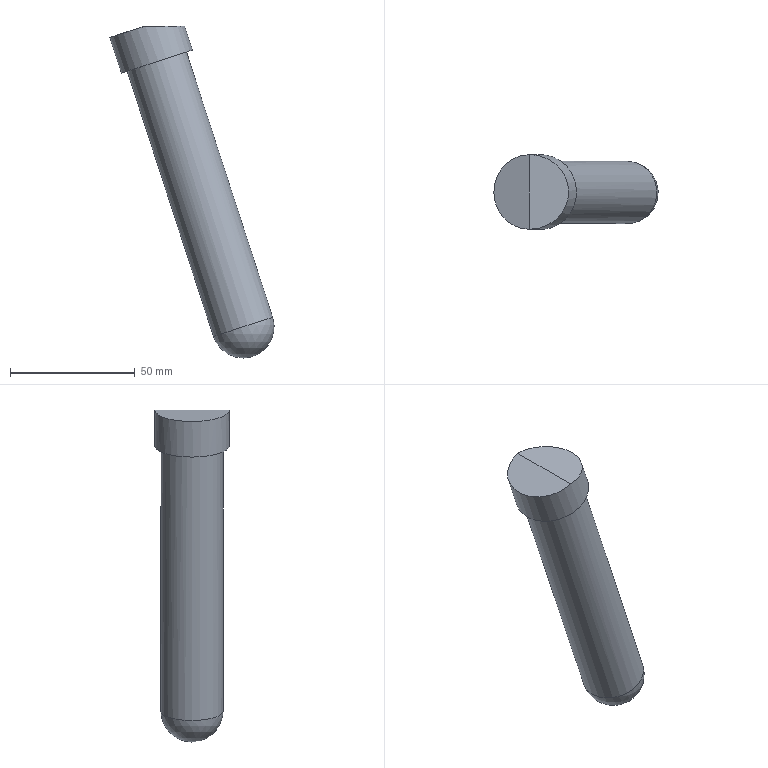Part | STEP file | solid 29 | 1 solid | 6 faces | box 66.011 x 30 x 133.284 mm | volume 68942 mm3 | plane 2 | cylinder 2 | spline 1 | sphere 1 | commonest cylinder face diameters 25 x1 30 x1